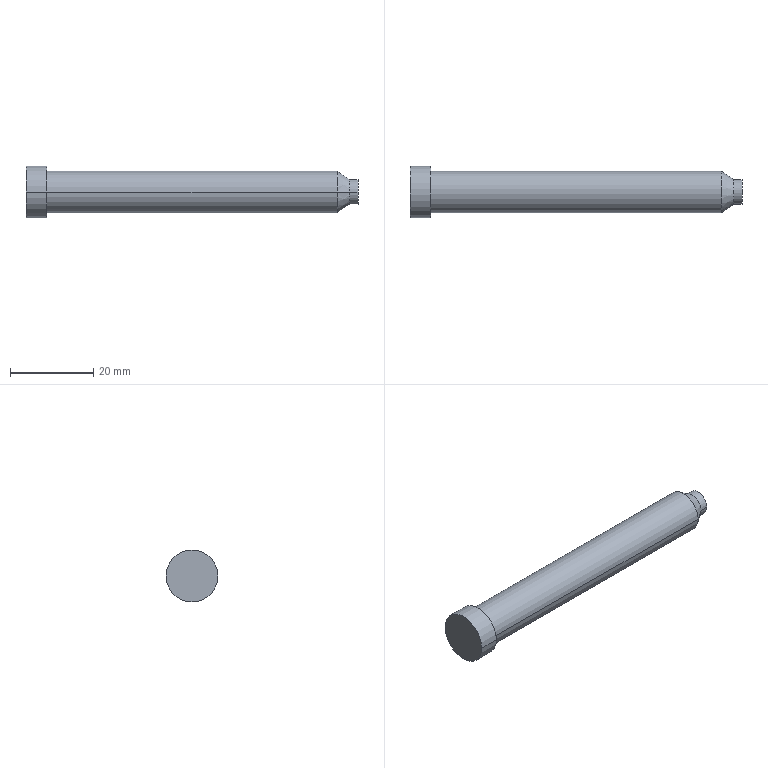Part | STEP file | CHOT DUC 6.0 | 1 solid | 11 faces | box 80 x 12.5 x 12.5 mm | volume 6322 mm3 | cylinder 6 | plane 3 | cone 2 | commonest cylinder face diameters 6 x2 10 x2 12.5 x2
STEP:
#1=CARTESIAN_POINT('',(0.,0.,0.));
#2=DIRECTION('',(0.,0.,1.));
#3=DIRECTION('',(1.,0.,0.));
#4=AXIS2_PLACEMENT_3D('',#1,#2,#3);
#5=CARTESIAN_POINT('',(-75.,5.,0.));
#6=VERTEX_POINT('',#5);
#7=CARTESIAN_POINT('',(-75.,-5.,0.));
#8=VERTEX_POINT('',#7);
#9=CARTESIAN_POINT('',(-75.,0.,0.));
#10=DIRECTION('',(1.,0.,0.));
#11=DIRECTION('',(0.,1.,0.));
#12=AXIS2_PLACEMENT_3D('',#9,#10,#11);
#13=CIRCLE('',#12,5.);
#14=CARTESIAN_POINT('',(-40.,0.,0.));
#15=DIRECTION('',(1.,0.,0.));
#16=DIRECTION('',(0.,1.,0.));
#17=AXIS2_PLACEMENT_3D('',#14,#15,#16);
#18=CYLINDRICAL_SURFACE('',#17,5.);
#19=CARTESIAN_POINT('',(0.,-35.));
#20=DIRECTION('',(1.,0.));
#21=VECTOR('',#20,1.);
#22=LINE('',#19,#21);
#23=(GEOMETRIC_REPRESENTATION_CONTEXT(2)PARAMETRIC_REPRESENTATION_CONTEXT()REPRESENTATION_CONTEXT('',''));
#24=DEFINITIONAL_REPRESENTATION('',(#22),#23);
#25=PCURVE('',#18,#24);
#26=CARTESIAN_POINT('',(-75.,5.625,0.));
#27=DIRECTION('',(1.,0.,0.));
#28=DIRECTION('',(0.,0.,-1.));
#29=AXIS2_PLACEMENT_3D('',#26,#27,#28);
#30=PLANE('',#29);
#31=CARTESIAN_POINT('',(0.,-5.625));
#32=DIRECTION('',(0.,1.));
#33=AXIS2_PLACEMENT_2D('',#31,#32);
#34=CIRCLE('',#33,5.);
#35=(GEOMETRIC_REPRESENTATION_CONTEXT(2)PARAMETRIC_REPRESENTATION_CONTEXT()REPRESENTATION_CONTEXT('',''));
#36=DEFINITIONAL_REPRESENTATION('',(#34),#35);
#37=PCURVE('',#30,#36);
#38=SURFACE_CURVE('',#13,(#25,#37),.PCURVE_S1.);
#39=EDGE_CURVE('',#6,#8,#38,.T.);
#40=ORIENTED_EDGE('',*,*,#39,.T.);
#41=CARTESIAN_POINT('',(-5.,-5.,0.));
#42=VERTEX_POINT('',#41);
#43=CARTESIAN_POINT('',(-40.,-5.,0.));
#44=DIRECTION('',(1.,0.,0.));
#45=VECTOR('',#44,1.);
#46=LINE('',#43,#45);
#47=CARTESIAN_POINT('',(3.142,0.));
#48=DIRECTION('',(0.,1.));
#49=VECTOR('',#48,1.);
#50=LINE('',#47,#49);
#51=(GEOMETRIC_REPRESENTATION_CONTEXT(2)PARAMETRIC_REPRESENTATION_CONTEXT()REPRESENTATION_CONTEXT('',''));
#52=DEFINITIONAL_REPRESENTATION('',(#50),#51);
#53=PCURVE('',#18,#52);
#54=CARTESIAN_POINT('',(-40.,0.,0.));
#55=DIRECTION('',(1.,0.,0.));
#56=DIRECTION('',(0.,1.,0.));
#57=AXIS2_PLACEMENT_3D('',#54,#55,#56);
#58=CYLINDRICAL_SURFACE('',#57,5.);
#59=CARTESIAN_POINT('',(3.142,0.));
#60=DIRECTION('',(0.,1.));
#61=VECTOR('',#60,1.);
#62=LINE('',#59,#61);
#63=(GEOMETRIC_REPRESENTATION_CONTEXT(2)PARAMETRIC_REPRESENTATION_CONTEXT()REPRESENTATION_CONTEXT('',''));
#64=DEFINITIONAL_REPRESENTATION('',(#62),#63);
#65=PCURVE('',#58,#64);
#66=SURFACE_CURVE('',#46,(#53,#65),.PCURVE_S1.);
#67=EDGE_CURVE('',#8,#42,#66,.T.);
#68=ORIENTED_EDGE('',*,*,#67,.T.);
#69=CARTESIAN_POINT('',(-5.,5.,0.));
#70=VERTEX_POINT('',#69);
#71=CARTESIAN_POINT('',(-5.,0.,0.));
#72=DIRECTION('',(-1.,0.,0.));
#73=DIRECTION('',(0.,1.,0.));
#74=AXIS2_PLACEMENT_3D('',#71,#72,#73);
#75=CIRCLE('',#74,5.);
#76=CARTESIAN_POINT('',(6.283,35.));
#77=DIRECTION('',(-1.,0.));
#78=VECTOR('',#77,1.);
#79=LINE('',#76,#78);
#80=(GEOMETRIC_REPRESENTATION_CONTEXT(2)PARAMETRIC_REPRESENTATION_CONTEXT()REPRESENTATION_CONTEXT('',''));
#81=DEFINITIONAL_REPRESENTATION('',(#79),#80);
#82=PCURVE('',#18,#81);
#83=CARTESIAN_POINT('',(-5.,0.,0.));
#84=DIRECTION('',(-1.,0.,0.));
#85=DIRECTION('',(0.,-1.,0.));
#86=AXIS2_PLACEMENT_3D('',#83,#84,#85);
#87=CONICAL_SURFACE('',#86,5.,0.588);
#88=CARTESIAN_POINT('',(-3.142,0.));
#89=DIRECTION('',(1.,0.));
#90=VECTOR('',#89,1.);
#91=LINE('',#88,#90);
#92=(GEOMETRIC_REPRESENTATION_CONTEXT(2)PARAMETRIC_REPRESENTATION_CONTEXT()REPRESENTATION_CONTEXT('',''));
#93=DEFINITIONAL_REPRESENTATION('',(#91),#92);
#94=PCURVE('',#87,#93);
#95=SURFACE_CURVE('',#75,(#82,#94),.PCURVE_S1.);
#96=EDGE_CURVE('',#42,#70,#95,.T.);
#97=ORIENTED_EDGE('',*,*,#96,.T.);
#98=CARTESIAN_POINT('',(-40.,5.,0.));
#99=DIRECTION('',(1.,0.,0.));
#100=VECTOR('',#99,1.);
#101=LINE('',#98,#100);
#102=CARTESIAN_POINT('',(0.,0.));
#103=DIRECTION('',(0.,1.));
#104=VECTOR('',#103,1.);
#105=LINE('',#102,#104);
#106=(GEOMETRIC_REPRESENTATION_CONTEXT(2)PARAMETRIC_REPRESENTATION_CONTEXT()REPRESENTATION_CONTEXT('',''));
#107=DEFINITIONAL_REPRESENTATION('',(#105),#106);
#108=PCURVE('',#18,#107);
#109=CARTESIAN_POINT('',(6.283,0.));
#110=DIRECTION('',(0.,1.));
#111=VECTOR('',#110,1.);
#112=LINE('',#109,#111);
#113=(GEOMETRIC_REPRESENTATION_CONTEXT(2)PARAMETRIC_REPRESENTATION_CONTEXT()REPRESENTATION_CONTEXT('',''));
#114=DEFINITIONAL_REPRESENTATION('',(#112),#113);
#115=PCURVE('',#58,#114);
#116=SURFACE_CURVE('',#101,(#108,#115),.PCURVE_S1.);
#117=EDGE_CURVE('',#6,#70,#116,.T.);
#118=ORIENTED_EDGE('',*,*,#117,.F.);
#119=EDGE_LOOP('',(#40,#68,#97,#118));
#120=FACE_BOUND('',#119,.T.);
#121=ADVANCED_FACE('',(#120),#18,.T.);
#122=CARTESIAN_POINT('',(-2.,-3.,0.));
#123=VERTEX_POINT('',#122);
#124=CARTESIAN_POINT('',(-2.,3.,0.));
#125=VERTEX_POINT('',#124);
#126=CARTESIAN_POINT('',(-2.,0.,0.));
#127=DIRECTION('',(-1.,0.,0.));
#128=DIRECTION('',(0.,1.,0.));
#129=AXIS2_PLACEMENT_3D('',#126,#127,#128);
#130=CIRCLE('',#129,3.);
#131=CARTESIAN_POINT('',(-3.142,-3.));
#132=DIRECTION('',(1.,0.));
#133=VECTOR('',#132,1.);
#134=LINE('',#131,#133);
#135=(GEOMETRIC_REPRESENTATION_CONTEXT(2)PARAMETRIC_REPRESENTATION_CONTEXT()REPRESENTATION_CONTEXT('',''));
#136=DEFINITIONAL_REPRESENTATION('',(#134),#135);
#137=PCURVE('',#87,#136);
#138=CARTESIAN_POINT('',(-1.,0.,0.));
#139=DIRECTION('',(1.,0.,0.));
#140=DIRECTION('',(0.,1.,0.));
#141=AXIS2_PLACEMENT_3D('',#138,#139,#140);
#142=CYLINDRICAL_SURFACE('',#141,3.);
#143=CARTESIAN_POINT('',(6.283,-1.));
#144=DIRECTION('',(-1.,0.));
#145=VECTOR('',#144,1.);
#146=LINE('',#143,#145);
#147=(GEOMETRIC_REPRESENTATION_CONTEXT(2)PARAMETRIC_REPRESENTATION_CONTEXT()REPRESENTATION_CONTEXT('',''));
#148=DEFINITIONAL_REPRESENTATION('',(#146),#147);
#149=PCURVE('',#142,#148);
#150=SURFACE_CURVE('',#130,(#137,#149),.PCURVE_S1.);
#151=EDGE_CURVE('',#123,#125,#150,.T.);
#152=ORIENTED_EDGE('',*,*,#151,.T.);
#153=CARTESIAN_POINT('',(-5.,5.,0.));
#154=DIRECTION('',(-0.8321,0.5547,0.));
#155=VECTOR('',#154,1.);
#156=LINE('',#153,#155);
#157=CARTESIAN_POINT('',(3.142,0.));
#158=DIRECTION('',(0.,1.));
#159=VECTOR('',#158,1.);
#160=LINE('',#157,#159);
#161=(GEOMETRIC_REPRESENTATION_CONTEXT(2)PARAMETRIC_REPRESENTATION_CONTEXT()REPRESENTATION_CONTEXT('',''));
#162=DEFINITIONAL_REPRESENTATION('',(#160),#161);
#163=PCURVE('',#87,#162);
#164=CARTESIAN_POINT('',(-5.,0.,0.));
#165=DIRECTION('',(-1.,0.,0.));
#166=DIRECTION('',(0.,-1.,0.));
#167=AXIS2_PLACEMENT_3D('',#164,#165,#166);
#168=CONICAL_SURFACE('',#167,5.,0.588);
#169=CARTESIAN_POINT('',(3.142,0.));
#170=DIRECTION('',(0.,1.));
#171=VECTOR('',#170,1.);
#172=LINE('',#169,#171);
#173=(GEOMETRIC_REPRESENTATION_CONTEXT(2)PARAMETRIC_REPRESENTATION_CONTEXT()REPRESENTATION_CONTEXT('',''));
#174=DEFINITIONAL_REPRESENTATION('',(#172),#173);
#175=PCURVE('',#168,#174);
#176=SURFACE_CURVE('',#156,(#163,#175),.PCURVE_S1.);
#177=EDGE_CURVE('',#125,#70,#176,.T.);
#178=ORIENTED_EDGE('',*,*,#177,.T.);
#179=ORIENTED_EDGE('',*,*,#96,.F.);
#180=CARTESIAN_POINT('',(-5.,-5.,0.));
#181=DIRECTION('',(-0.8321,-0.5547,0.));
#182=VECTOR('',#181,1.);
#183=LINE('',#180,#182);
#184=CARTESIAN_POINT('',(0.,0.));
#185=DIRECTION('',(0.,1.));
#186=VECTOR('',#185,1.);
#187=LINE('',#184,#186);
#188=(GEOMETRIC_REPRESENTATION_CONTEXT(2)PARAMETRIC_REPRESENTATION_CONTEXT()REPRESENTATION_CONTEXT('',''));
#189=DEFINITIONAL_REPRESENTATION('',(#187),#188);
#190=PCURVE('',#87,#189);
#191=CARTESIAN_POINT('',(6.283,0.));
#192=DIRECTION('',(0.,1.));
#193=VECTOR('',#192,1.);
#194=LINE('',#191,#193);
#195=(GEOMETRIC_REPRESENTATION_CONTEXT(2)PARAMETRIC_REPRESENTATION_CONTEXT()REPRESENTATION_CONTEXT('',''));
#196=DEFINITIONAL_REPRESENTATION('',(#194),#195);
#197=PCURVE('',#168,#196);
#198=SURFACE_CURVE('',#183,(#190,#197),.PCURVE_S1.);
#199=EDGE_CURVE('',#123,#42,#198,.T.);
#200=ORIENTED_EDGE('',*,*,#199,.F.);
#201=EDGE_LOOP('',(#152,#178,#179,#200));
#202=FACE_BOUND('',#201,.T.);
#203=ADVANCED_FACE('',(#202),#87,.T.);
#204=CARTESIAN_POINT('',(-80.,6.25,0.));
#205=VERTEX_POINT('',#204);
#206=CARTESIAN_POINT('',(-80.,-6.25,0.));
#207=VERTEX_POINT('',#206);
#208=CARTESIAN_POINT('',(-80.,0.,0.));
#209=DIRECTION('',(1.,0.,0.));
#210=DIRECTION('',(0.,1.,0.));
#211=AXIS2_PLACEMENT_3D('',#208,#209,#210);
#212=CIRCLE('',#211,6.25);
#213=CARTESIAN_POINT('',(-77.5,0.,0.));
#214=DIRECTION('',(1.,0.,0.));
#215=DIRECTION('',(0.,1.,0.));
#216=AXIS2_PLACEMENT_3D('',#213,#214,#215);
#217=CYLINDRICAL_SURFACE('',#216,6.25);
#218=CARTESIAN_POINT('',(0.,-2.5));
#219=DIRECTION('',(1.,0.));
#220=VECTOR('',#219,1.);
#221=LINE('',#218,#220);
#222=(GEOMETRIC_REPRESENTATION_CONTEXT(2)PARAMETRIC_REPRESENTATION_CONTEXT()REPRESENTATION_CONTEXT('',''));
#223=DEFINITIONAL_REPRESENTATION('',(#221),#222);
#224=PCURVE('',#217,#223);
#225=CARTESIAN_POINT('',(-80.,3.125,0.));
#226=DIRECTION('',(-1.,0.,0.));
#227=DIRECTION('',(0.,0.,1.));
#228=AXIS2_PLACEMENT_3D('',#225,#226,#227);
#229=PLANE('',#228);
#230=CARTESIAN_POINT('',(0.,3.125));
#231=CARTESIAN_POINT('',(10.825,3.125));
#232=CARTESIAN_POINT('',(5.413,-6.25));
#233=CARTESIAN_POINT('',(0.,-15.625));
#234=CARTESIAN_POINT('',(-5.413,-6.25));
#235=CARTESIAN_POINT('',(-10.825,3.125));
#236=CARTESIAN_POINT('',(0.,3.125));
#237=(BOUNDED_CURVE()B_SPLINE_CURVE(2,(#230,#231,#232,#233,#234,#235,#236),.UNSPECIFIED.,.T.,.F.)B_SPLINE_CURVE_WITH_KNOTS((1,2,2,2,2,1),(-2.094,0.,2.094,4.189,6.283,8.378),.UNSPECIFIED.)CURVE()GEOMETRIC_REPRESENTATION_ITEM()RATIONAL_B_SPLINE_CURVE((1.,0.5,1.,0.5,1.,0.5,1.))REPRESENTATION_ITEM(''));
#238=(GEOMETRIC_REPRESENTATION_CONTEXT(2)PARAMETRIC_REPRESENTATION_CONTEXT()REPRESENTATION_CONTEXT('',''));
#239=DEFINITIONAL_REPRESENTATION('',(#237),#238);
#240=PCURVE('',#229,#239);
#241=SURFACE_CURVE('',#212,(#224,#240),.PCURVE_S1.);
#242=EDGE_CURVE('',#205,#207,#241,.T.);
#243=ORIENTED_EDGE('',*,*,#242,.T.);
#244=CARTESIAN_POINT('',(-75.,-6.25,0.));
#245=VERTEX_POINT('',#244);
#246=CARTESIAN_POINT('',(-77.5,-6.25,0.));
#247=DIRECTION('',(1.,0.,0.));
#248=VECTOR('',#247,1.);
#249=LINE('',#246,#248);
#250=CARTESIAN_POINT('',(3.142,0.));
#251=DIRECTION('',(0.,1.));
#252=VECTOR('',#251,1.);
#253=LINE('',#250,#252);
#254=(GEOMETRIC_REPRESENTATION_CONTEXT(2)PARAMETRIC_REPRESENTATION_CONTEXT()REPRESENTATION_CONTEXT('',''));
#255=DEFINITIONAL_REPRESENTATION('',(#253),#254);
#256=PCURVE('',#217,#255);
#257=CARTESIAN_POINT('',(-77.5,0.,0.));
#258=DIRECTION('',(1.,0.,0.));
#259=DIRECTION('',(0.,1.,0.));
#260=AXIS2_PLACEMENT_3D('',#257,#258,#259);
#261=CYLINDRICAL_SURFACE('',#260,6.25);
#262=CARTESIAN_POINT('',(3.142,0.));
#263=DIRECTION('',(0.,1.));
#264=VECTOR('',#263,1.);
#265=LINE('',#262,#264);
#266=(GEOMETRIC_REPRESENTATION_CONTEXT(2)PARAMETRIC_REPRESENTATION_CONTEXT()REPRESENTATION_CONTEXT('',''));
#267=DEFINITIONAL_REPRESENTATION('',(#265),#266);
#268=PCURVE('',#261,#267);
#269=SURFACE_CURVE('',#249,(#256,#268),.PCURVE_S1.);
#270=EDGE_CURVE('',#207,#245,#269,.T.);
#271=ORIENTED_EDGE('',*,*,#270,.T.);
#272=CARTESIAN_POINT('',(-75.,6.25,0.));
#273=VERTEX_POINT('',#272);
#274=CARTESIAN_POINT('',(-75.,0.,0.));
#275=DIRECTION('',(1.,0.,0.));
#276=DIRECTION('',(0.,1.,0.));
#277=AXIS2_PLACEMENT_3D('',#274,#275,#276);
#278=CIRCLE('',#277,6.25);
#279=CARTESIAN_POINT('',(0.,2.5));
#280=DIRECTION('',(1.,0.));
#281=VECTOR('',#280,1.);
#282=LINE('',#279,#281);
#283=(GEOMETRIC_REPRESENTATION_CONTEXT(2)PARAMETRIC_REPRESENTATION_CONTEXT()REPRESENTATION_CONTEXT('',''));
#284=DEFINITIONAL_REPRESENTATION('',(#282),#283);
#285=PCURVE('',#217,#284);
#286=CARTESIAN_POINT('',(0.,-5.625));
#287=DIRECTION('',(0.,1.));
#288=AXIS2_PLACEMENT_2D('',#286,#287);
#289=CIRCLE('',#288,6.25);
#290=(GEOMETRIC_REPRESENTATION_CONTEXT(2)PARAMETRIC_REPRESENTATION_CONTEXT()REPRESENTATION_CONTEXT('',''));
#291=DEFINITIONAL_REPRESENTATION('',(#289),#290);
#292=PCURVE('',#30,#291);
#293=SURFACE_CURVE('',#278,(#285,#292),.PCURVE_S1.);
#294=EDGE_CURVE('',#273,#245,#293,.T.);
#295=ORIENTED_EDGE('',*,*,#294,.F.);
#296=CARTESIAN_POINT('',(-77.5,6.25,0.));
#297=DIRECTION('',(1.,0.,0.));
#298=VECTOR('',#297,1.);
#299=LINE('',#296,#298);
#300=CARTESIAN_POINT('',(0.,0.));
#301=DIRECTION('',(0.,1.));
#302=VECTOR('',#301,1.);
#303=LINE('',#300,#302);
#304=(GEOMETRIC_REPRESENTATION_CONTEXT(2)PARAMETRIC_REPRESENTATION_CONTEXT()REPRESENTATION_CONTEXT('',''));
#305=DEFINITIONAL_REPRESENTATION('',(#303),#304);
#306=PCURVE('',#217,#305);
#307=CARTESIAN_POINT('',(6.283,0.));
#308=DIRECTION('',(0.,1.));
#309=VECTOR('',#308,1.);
#310=LINE('',#307,#309);
#311=(GEOMETRIC_REPRESENTATION_CONTEXT(2)PARAMETRIC_REPRESENTATION_CONTEXT()REPRESENTATION_CONTEXT('',''));
#312=DEFINITIONAL_REPRESENTATION('',(#310),#311);
#313=PCURVE('',#261,#312);
#314=SURFACE_CURVE('',#299,(#306,#313),.PCURVE_S1.);
#315=EDGE_CURVE('',#205,#273,#314,.T.);
#316=ORIENTED_EDGE('',*,*,#315,.F.);
#317=EDGE_LOOP('',(#243,#271,#295,#316));
#318=FACE_BOUND('',#317,.T.);
#319=ADVANCED_FACE('',(#318),#217,.T.);
#320=ORIENTED_EDGE('',*,*,#151,.F.);
#321=CARTESIAN_POINT('',(0.,-3.,0.));
#322=VERTEX_POINT('',#321);
#323=CARTESIAN_POINT('',(-1.,-3.,0.));
#324=DIRECTION('',(1.,0.,0.));
#325=VECTOR('',#324,1.);
#326=LINE('',#323,#325);
#327=CARTESIAN_POINT('',(3.142,0.));
#328=DIRECTION('',(0.,1.));
#329=VECTOR('',#328,1.);
#330=LINE('',#327,#329);
#331=(GEOMETRIC_REPRESENTATION_CONTEXT(2)PARAMETRIC_REPRESENTATION_CONTEXT()REPRESENTATION_CONTEXT('',''));
#332=DEFINITIONAL_REPRESENTATION('',(#330),#331);
#333=PCURVE('',#142,#332);
#334=CARTESIAN_POINT('',(-1.,0.,0.));
#335=DIRECTION('',(1.,0.,0.));
#336=DIRECTION('',(0.,1.,0.));
#337=AXIS2_PLACEMENT_3D('',#334,#335,#336);
#338=CYLINDRICAL_SURFACE('',#337,3.);
#339=CARTESIAN_POINT('',(3.142,0.));
#340=DIRECTION('',(0.,1.));
#341=VECTOR('',#340,1.);
#342=LINE('',#339,#341);
#343=(GEOMETRIC_REPRESENTATION_CONTEXT(2)PARAMETRIC_REPRESENTATION_CONTEXT()REPRESENTATION_CONTEXT('',''));
#344=DEFINITIONAL_REPRESENTATION('',(#342),#343);
#345=PCURVE('',#338,#344);
#346=SURFACE_CURVE('',#326,(#333,#345),.PCURVE_S1.);
#347=EDGE_CURVE('',#123,#322,#346,.T.);
#348=ORIENTED_EDGE('',*,*,#347,.T.);
#349=CARTESIAN_POINT('',(0.,3.,0.));
#350=VERTEX_POINT('',#349);
#351=CARTESIAN_POINT('',(0.,0.,0.));
#352=DIRECTION('',(-1.,0.,0.));
#353=DIRECTION('',(0.,1.,0.));
#354=AXIS2_PLACEMENT_3D('',#351,#352,#353);
#355=CIRCLE('',#354,3.);
#356=CARTESIAN_POINT('',(6.283,1.));
#357=DIRECTION('',(-1.,0.));
#358=VECTOR('',#357,1.);
#359=LINE('',#356,#358);
#360=(GEOMETRIC_REPRESENTATION_CONTEXT(2)PARAMETRIC_REPRESENTATION_CONTEXT()REPRESENTATION_CONTEXT('',''));
#361=DEFINITIONAL_REPRESENTATION('',(#359),#360);
#362=PCURVE('',#142,#361);
#363=CARTESIAN_POINT('',(0.,1.5,0.));
#364=DIRECTION('',(1.,0.,0.));
#365=DIRECTION('',(0.,0.,-1.));
#366=AXIS2_PLACEMENT_3D('',#363,#364,#365);
#367=PLANE('',#366);
#368=CARTESIAN_POINT('',(0.,1.5));
#369=CARTESIAN_POINT('',(5.196,1.5));
#370=CARTESIAN_POINT('',(2.598,-3.));
#371=CARTESIAN_POINT('',(0.,-7.5));
#372=CARTESIAN_POINT('',(-2.598,-3.));
#373=CARTESIAN_POINT('',(-5.196,1.5));
#374=CARTESIAN_POINT('',(0.,1.5));
#375=(BOUNDED_CURVE()B_SPLINE_CURVE(2,(#368,#369,#370,#371,#372,#373,#374),.UNSPECIFIED.,.T.,.F.)B_SPLINE_CURVE_WITH_KNOTS((1,2,2,2,2,1),(-2.094,0.,2.094,4.189,6.283,8.378),.UNSPECIFIED.)CURVE()GEOMETRIC_REPRESENTATION_ITEM()RATIONAL_B_SPLINE_CURVE((1.,0.5,1.,0.5,1.,0.5,1.))REPRESENTATION_ITEM(''));
#376=(GEOMETRIC_REPRESENTATION_CONTEXT(2)PARAMETRIC_REPRESENTATION_CONTEXT()REPRESENTATION_CONTEXT('',''));
#377=DEFINITIONAL_REPRESENTATION('',(#375),#376);
#378=PCURVE('',#367,#377);
#379=SURFACE_CURVE('',#355,(#362,#378),.PCURVE_S1.);
#380=EDGE_CURVE('',#322,#350,#379,.T.);
#381=ORIENTED_EDGE('',*,*,#380,.T.);
#382=CARTESIAN_POINT('',(-1.,3.,0.));
#383=DIRECTION('',(1.,0.,0.));
#384=VECTOR('',#383,1.);
#385=LINE('',#382,#384);
#386=CARTESIAN_POINT('',(0.,0.));
#387=DIRECTION('',(0.,1.));
#388=VECTOR('',#387,1.);
#389=LINE('',#386,#388);
#390=(GEOMETRIC_REPRESENTATION_CONTEXT(2)PARAMETRIC_REPRESENTATION_CONTEXT()REPRESENTATION_CONTEXT('',''));
#391=DEFINITIONAL_REPRESENTATION('',(#389),#390);
#392=PCURVE('',#142,#391);
#393=CARTESIAN_POINT('',(6.283,0.));
#394=DIRECTION('',(0.,1.));
#395=VECTOR('',#394,1.);
#396=LINE('',#393,#395);
#397=(GEOMETRIC_REPRESENTATION_CONTEXT(2)PARAMETRIC_REPRESENTATION_CONTEXT()REPRESENTATION_CONTEXT('',''));
#398=DEFINITIONAL_REPRESENTATION('',(#396),#397);
#399=PCURVE('',#338,#398);
#400=SURFACE_CURVE('',#385,(#392,#399),.PCURVE_S1.);
#401=EDGE_CURVE('',#125,#350,#400,.T.);
#402=ORIENTED_EDGE('',*,*,#401,.F.);
#403=EDGE_LOOP('',(#320,#348,#381,#402));
#404=FACE_BOUND('',#403,.T.);
#405=ADVANCED_FACE('',(#404),#142,.T.);
#406=ORIENTED_EDGE('',*,*,#67,.F.);
#407=CARTESIAN_POINT('',(-75.,0.,0.));
#408=DIRECTION('',(1.,0.,0.));
#409=DIRECTION('',(0.,1.,0.));
#410=AXIS2_PLACEMENT_3D('',#407,#408,#409);
#411=CIRCLE('',#410,5.);
#412=CARTESIAN_POINT('',(0.,-35.));
#413=DIRECTION('',(1.,0.));
#414=VECTOR('',#413,1.);
#415=LINE('',#412,#414);
#416=(GEOMETRIC_REPRESENTATION_CONTEXT(2)PARAMETRIC_REPRESENTATION_CONTEXT()REPRESENTATION_CONTEXT('',''));
#417=DEFINITIONAL_REPRESENTATION('',(#415),#416);
#418=PCURVE('',#58,#417);
#419=CARTESIAN_POINT('',(0.,-5.625));
#420=DIRECTION('',(0.,1.));
#421=AXIS2_PLACEMENT_2D('',#419,#420);
#422=CIRCLE('',#421,5.);
#423=(GEOMETRIC_REPRESENTATION_CONTEXT(2)PARAMETRIC_REPRESENTATION_CONTEXT()REPRESENTATION_CONTEXT('',''));
#424=DEFINITIONAL_REPRESENTATION('',(#422),#423);
#425=PCURVE('',#30,#424);
#426=SURFACE_CURVE('',#411,(#418,#425),.PCURVE_S1.);
#427=EDGE_CURVE('',#8,#6,#426,.T.);
#428=ORIENTED_EDGE('',*,*,#427,.T.);
#429=ORIENTED_EDGE('',*,*,#117,.T.);
#430=CARTESIAN_POINT('',(-5.,0.,0.));
#431=DIRECTION('',(-1.,0.,0.));
#432=DIRECTION('',(0.,1.,0.));
#433=AXIS2_PLACEMENT_3D('',#430,#431,#432);
#434=CIRCLE('',#433,5.);
#435=CARTESIAN_POINT('',(6.283,35.));
#436=DIRECTION('',(-1.,0.));
#437=VECTOR('',#436,1.);
#438=LINE('',#435,#437);
#439=(GEOMETRIC_REPRESENTATION_CONTEXT(2)PARAMETRIC_REPRESENTATION_CONTEXT()REPRESENTATION_CONTEXT('',''));
#440=DEFINITIONAL_REPRESENTATION('',(#438),#439);
#441=PCURVE('',#58,#440);
#442=CARTESIAN_POINT('',(3.142,0.));
#443=DIRECTION('',(1.,0.));
#444=VECTOR('',#443,1.);
#445=LINE('',#442,#444);
#446=(GEOMETRIC_REPRESENTATION_CONTEXT(2)PARAMETRIC_REPRESENTATION_CONTEXT()REPRESENTATION_CONTEXT('',''));
#447=DEFINITIONAL_REPRESENTATION('',(#445),#446);
#448=PCURVE('',#168,#447);
#449=SURFACE_CURVE('',#434,(#441,#448),.PCURVE_S1.);
#450=EDGE_CURVE('',#70,#42,#449,.T.);
#451=ORIENTED_EDGE('',*,*,#450,.T.);
#452=EDGE_LOOP('',(#406,#428,#429,#451));
#453=FACE_BOUND('',#452,.T.);
#454=ADVANCED_FACE('',(#453),#58,.T.);
#455=ORIENTED_EDGE('',*,*,#39,.F.);
#456=ORIENTED_EDGE('',*,*,#427,.F.);
#457=EDGE_LOOP('',(#455,#456));
#458=FACE_BOUND('',#457,.T.);
#459=ORIENTED_EDGE('',*,*,#294,.T.);
#460=CARTESIAN_POINT('',(-75.,0.,0.));
#461=DIRECTION('',(1.,0.,0.));
#462=DIRECTION('',(0.,1.,0.));
#463=AXIS2_PLACEMENT_3D('',#460,#461,#462);
#464=CIRCLE('',#463,6.25);
#465=CARTESIAN_POINT('',(0.,-5.625));
#466=DIRECTION('',(0.,1.));
#467=AXIS2_PLACEMENT_2D('',#465,#466);
#468=CIRCLE('',#467,6.25);
#469=(GEOMETRIC_REPRESENTATION_CONTEXT(2)PARAMETRIC_REPRESENTATION_CONTEXT()REPRESENTATION_CONTEXT('',''));
#470=DEFINITIONAL_REPRESENTATION('',(#468),#469);
#471=PCURVE('',#30,#470);
#472=CARTESIAN_POINT('',(0.,2.5));
#473=DIRECTION('',(1.,0.));
#474=VECTOR('',#473,1.);
#475=LINE('',#472,#474);
#476=(GEOMETRIC_REPRESENTATION_CONTEXT(2)PARAMETRIC_REPRESENTATION_CONTEXT()REPRESENTATION_CONTEXT('',''));
#477=DEFINITIONAL_REPRESENTATION('',(#475),#476);
#478=PCURVE('',#261,#477);
#479=SURFACE_CURVE('',#464,(#471,#478),.PCURVE_S1.);
#480=EDGE_CURVE('',#245,#273,#479,.T.);
#481=ORIENTED_EDGE('',*,*,#480,.T.);
#482=EDGE_LOOP('',(#459,#481));
#483=FACE_BOUND('',#482,.T.);
#484=ADVANCED_FACE('',(#458,#483),#30,.T.);
#485=ORIENTED_EDGE('',*,*,#177,.F.);
#486=CARTESIAN_POINT('',(-2.,0.,0.));
#487=DIRECTION('',(-1.,0.,0.));
#488=DIRECTION('',(0.,1.,0.));
#489=AXIS2_PLACEMENT_3D('',#486,#487,#488);
#490=CIRCLE('',#489,3.);
#491=CARTESIAN_POINT('',(3.142,-3.));
#492=DIRECTION('',(1.,0.));
#493=VECTOR('',#492,1.);
#494=LINE('',#491,#493);
#495=(GEOMETRIC_REPRESENTATION_CONTEXT(2)PARAMETRIC_REPRESENTATION_CONTEXT()REPRESENTATION_CONTEXT('',''));
#496=DEFINITIONAL_REPRESENTATION('',(#494),#495);
#497=PCURVE('',#168,#496);
#498=CARTESIAN_POINT('',(6.283,-1.));
#499=DIRECTION('',(-1.,0.));
#500=VECTOR('',#499,1.);
#501=LINE('',#498,#500);
#502=(GEOMETRIC_REPRESENTATION_CONTEXT(2)PARAMETRIC_REPRESENTATION_CONTEXT()REPRESENTATION_CONTEXT('',''));
#503=DEFINITIONAL_REPRESENTATION('',(#501),#502);
#504=PCURVE('',#338,#503);
#505=SURFACE_CURVE('',#490,(#497,#504),.PCURVE_S1.);
#506=EDGE_CURVE('',#125,#123,#505,.T.);
#507=ORIENTED_EDGE('',*,*,#506,.T.);
#508=ORIENTED_EDGE('',*,*,#199,.T.);
#509=ORIENTED_EDGE('',*,*,#450,.F.);
#510=EDGE_LOOP('',(#485,#507,#508,#509));
#511=FACE_BOUND('',#510,.T.);
#512=ADVANCED_FACE('',(#511),#168,.T.);
#513=ORIENTED_EDGE('',*,*,#270,.F.);
#514=CARTESIAN_POINT('',(-80.,0.,0.));
#515=DIRECTION('',(1.,0.,0.));
#516=DIRECTION('',(0.,1.,0.));
#517=AXIS2_PLACEMENT_3D('',#514,#515,#516);
#518=CIRCLE('',#517,6.25);
#519=CARTESIAN_POINT('',(0.,-2.5));
#520=DIRECTION('',(1.,0.));
#521=VECTOR('',#520,1.);
#522=LINE('',#519,#521);
#523=(GEOMETRIC_REPRESENTATION_CONTEXT(2)PARAMETRIC_REPRESENTATION_CONTEXT()REPRESENTATION_CONTEXT('',''));
#524=DEFINITIONAL_REPRESENTATION('',(#522),#523);
#525=PCURVE('',#261,#524);
#526=CARTESIAN_POINT('',(0.,3.125));
#527=CARTESIAN_POINT('',(10.825,3.125));
#528=CARTESIAN_POINT('',(5.413,-6.25));
#529=CARTESIAN_POINT('',(0.,-15.625));
#530=CARTESIAN_POINT('',(-5.413,-6.25));
#531=CARTESIAN_POINT('',(-10.825,3.125));
#532=CARTESIAN_POINT('',(0.,3.125));
#533=(BOUNDED_CURVE()B_SPLINE_CURVE(2,(#526,#527,#528,#529,#530,#531,#532),.UNSPECIFIED.,.T.,.F.)B_SPLINE_CURVE_WITH_KNOTS((1,2,2,2,2,1),(-2.094,0.,2.094,4.189,6.283,8.378),.UNSPECIFIED.)CURVE()GEOMETRIC_REPRESENTATION_ITEM()RATIONAL_B_SPLINE_CURVE((1.,0.5,1.,0.5,1.,0.5,1.))REPRESENTATION_ITEM(''));
#534=(GEOMETRIC_REPRESENTATION_CONTEXT(2)PARAMETRIC_REPRESENTATION_CONTEXT()REPRESENTATION_CONTEXT('',''));
#535=DEFINITIONAL_REPRESENTATION('',(#533),#534);
#536=PCURVE('',#229,#535);
#537=SURFACE_CURVE('',#518,(#525,#536),.PCURVE_S1.);
#538=EDGE_CURVE('',#207,#205,#537,.T.);
#539=ORIENTED_EDGE('',*,*,#538,.T.);
#540=ORIENTED_EDGE('',*,*,#315,.T.);
#541=ORIENTED_EDGE('',*,*,#480,.F.);
#542=EDGE_LOOP('',(#513,#539,#540,#541));
#543=FACE_BOUND('',#542,.T.);
#544=ADVANCED_FACE('',(#543),#261,.T.);
#545=ORIENTED_EDGE('',*,*,#347,.F.);
#546=ORIENTED_EDGE('',*,*,#506,.F.);
#547=ORIENTED_EDGE('',*,*,#401,.T.);
#548=CARTESIAN_POINT('',(0.,0.,0.));
#549=DIRECTION('',(-1.,0.,0.));
#550=DIRECTION('',(0.,1.,0.));
#551=AXIS2_PLACEMENT_3D('',#548,#549,#550);
#552=CIRCLE('',#551,3.);
#553=CARTESIAN_POINT('',(6.283,1.));
#554=DIRECTION('',(-1.,0.));
#555=VECTOR('',#554,1.);
#556=LINE('',#553,#555);
#557=(GEOMETRIC_REPRESENTATION_CONTEXT(2)PARAMETRIC_REPRESENTATION_CONTEXT()REPRESENTATION_CONTEXT('',''));
#558=DEFINITIONAL_REPRESENTATION('',(#556),#557);
#559=PCURVE('',#338,#558);
#560=CARTESIAN_POINT('',(0.,1.5));
#561=CARTESIAN_POINT('',(5.196,1.5));
#562=CARTESIAN_POINT('',(2.598,-3.));
#563=CARTESIAN_POINT('',(0.,-7.5));
#564=CARTESIAN_POINT('',(-2.598,-3.));
#565=CARTESIAN_POINT('',(-5.196,1.5));
#566=CARTESIAN_POINT('',(0.,1.5));
#567=(BOUNDED_CURVE()B_SPLINE_CURVE(2,(#560,#561,#562,#563,#564,#565,#566),.UNSPECIFIED.,.T.,.F.)B_SPLINE_CURVE_WITH_KNOTS((1,2,2,2,2,1),(-2.094,0.,2.094,4.189,6.283,8.378),.UNSPECIFIED.)CURVE()GEOMETRIC_REPRESENTATION_ITEM()RATIONAL_B_SPLINE_CURVE((1.,0.5,1.,0.5,1.,0.5,1.))REPRESENTATION_ITEM(''));
#568=(GEOMETRIC_REPRESENTATION_CONTEXT(2)PARAMETRIC_REPRESENTATION_CONTEXT()REPRESENTATION_CONTEXT('',''));
#569=DEFINITIONAL_REPRESENTATION('',(#567),#568);
#570=PCURVE('',#367,#569);
#571=SURFACE_CURVE('',#552,(#559,#570),.PCURVE_S1.);
#572=EDGE_CURVE('',#350,#322,#571,.T.);
#573=ORIENTED_EDGE('',*,*,#572,.T.);
#574=EDGE_LOOP('',(#545,#546,#547,#573));
#575=FACE_BOUND('',#574,.T.);
#576=ADVANCED_FACE('',(#575),#338,.T.);
#577=ORIENTED_EDGE('',*,*,#242,.F.);
#578=ORIENTED_EDGE('',*,*,#538,.F.);
#579=EDGE_LOOP('',(#577,#578));
#580=FACE_BOUND('',#579,.T.);
#581=ADVANCED_FACE('',(#580),#229,.T.);
#582=ORIENTED_EDGE('',*,*,#572,.F.);
#583=ORIENTED_EDGE('',*,*,#380,.F.);
#584=EDGE_LOOP('',(#582,#583));
#585=FACE_BOUND('',#584,.T.);
#586=ADVANCED_FACE('',(#585),#367,.T.);
#587=CLOSED_SHELL('',(#121,#203,#319,#405,#454,#484,#512,#544,#576,#581,#586));
#588=MANIFOLD_SOLID_BREP('',#587);
#589=(LENGTH_UNIT()NAMED_UNIT(*)SI_UNIT(.MILLI.,.METRE.));
#590=UNCERTAINTY_MEASURE_WITH_UNIT(LENGTH_MEASURE(0.0000001),#589,'','');
#591=(NAMED_UNIT(*)PLANE_ANGLE_UNIT()SI_UNIT($,.RADIAN.));
#592=(NAMED_UNIT(*)SI_UNIT($,.STERADIAN.)SOLID_ANGLE_UNIT());
#593=(GEOMETRIC_REPRESENTATION_CONTEXT(3)GLOBAL_UNCERTAINTY_ASSIGNED_CONTEXT((#590))GLOBAL_UNIT_ASSIGNED_CONTEXT((#589,#591,#592))REPRESENTATION_CONTEXT('',''));
#594=ADVANCED_BREP_SHAPE_REPRESENTATION('',(#4,#588),#593);